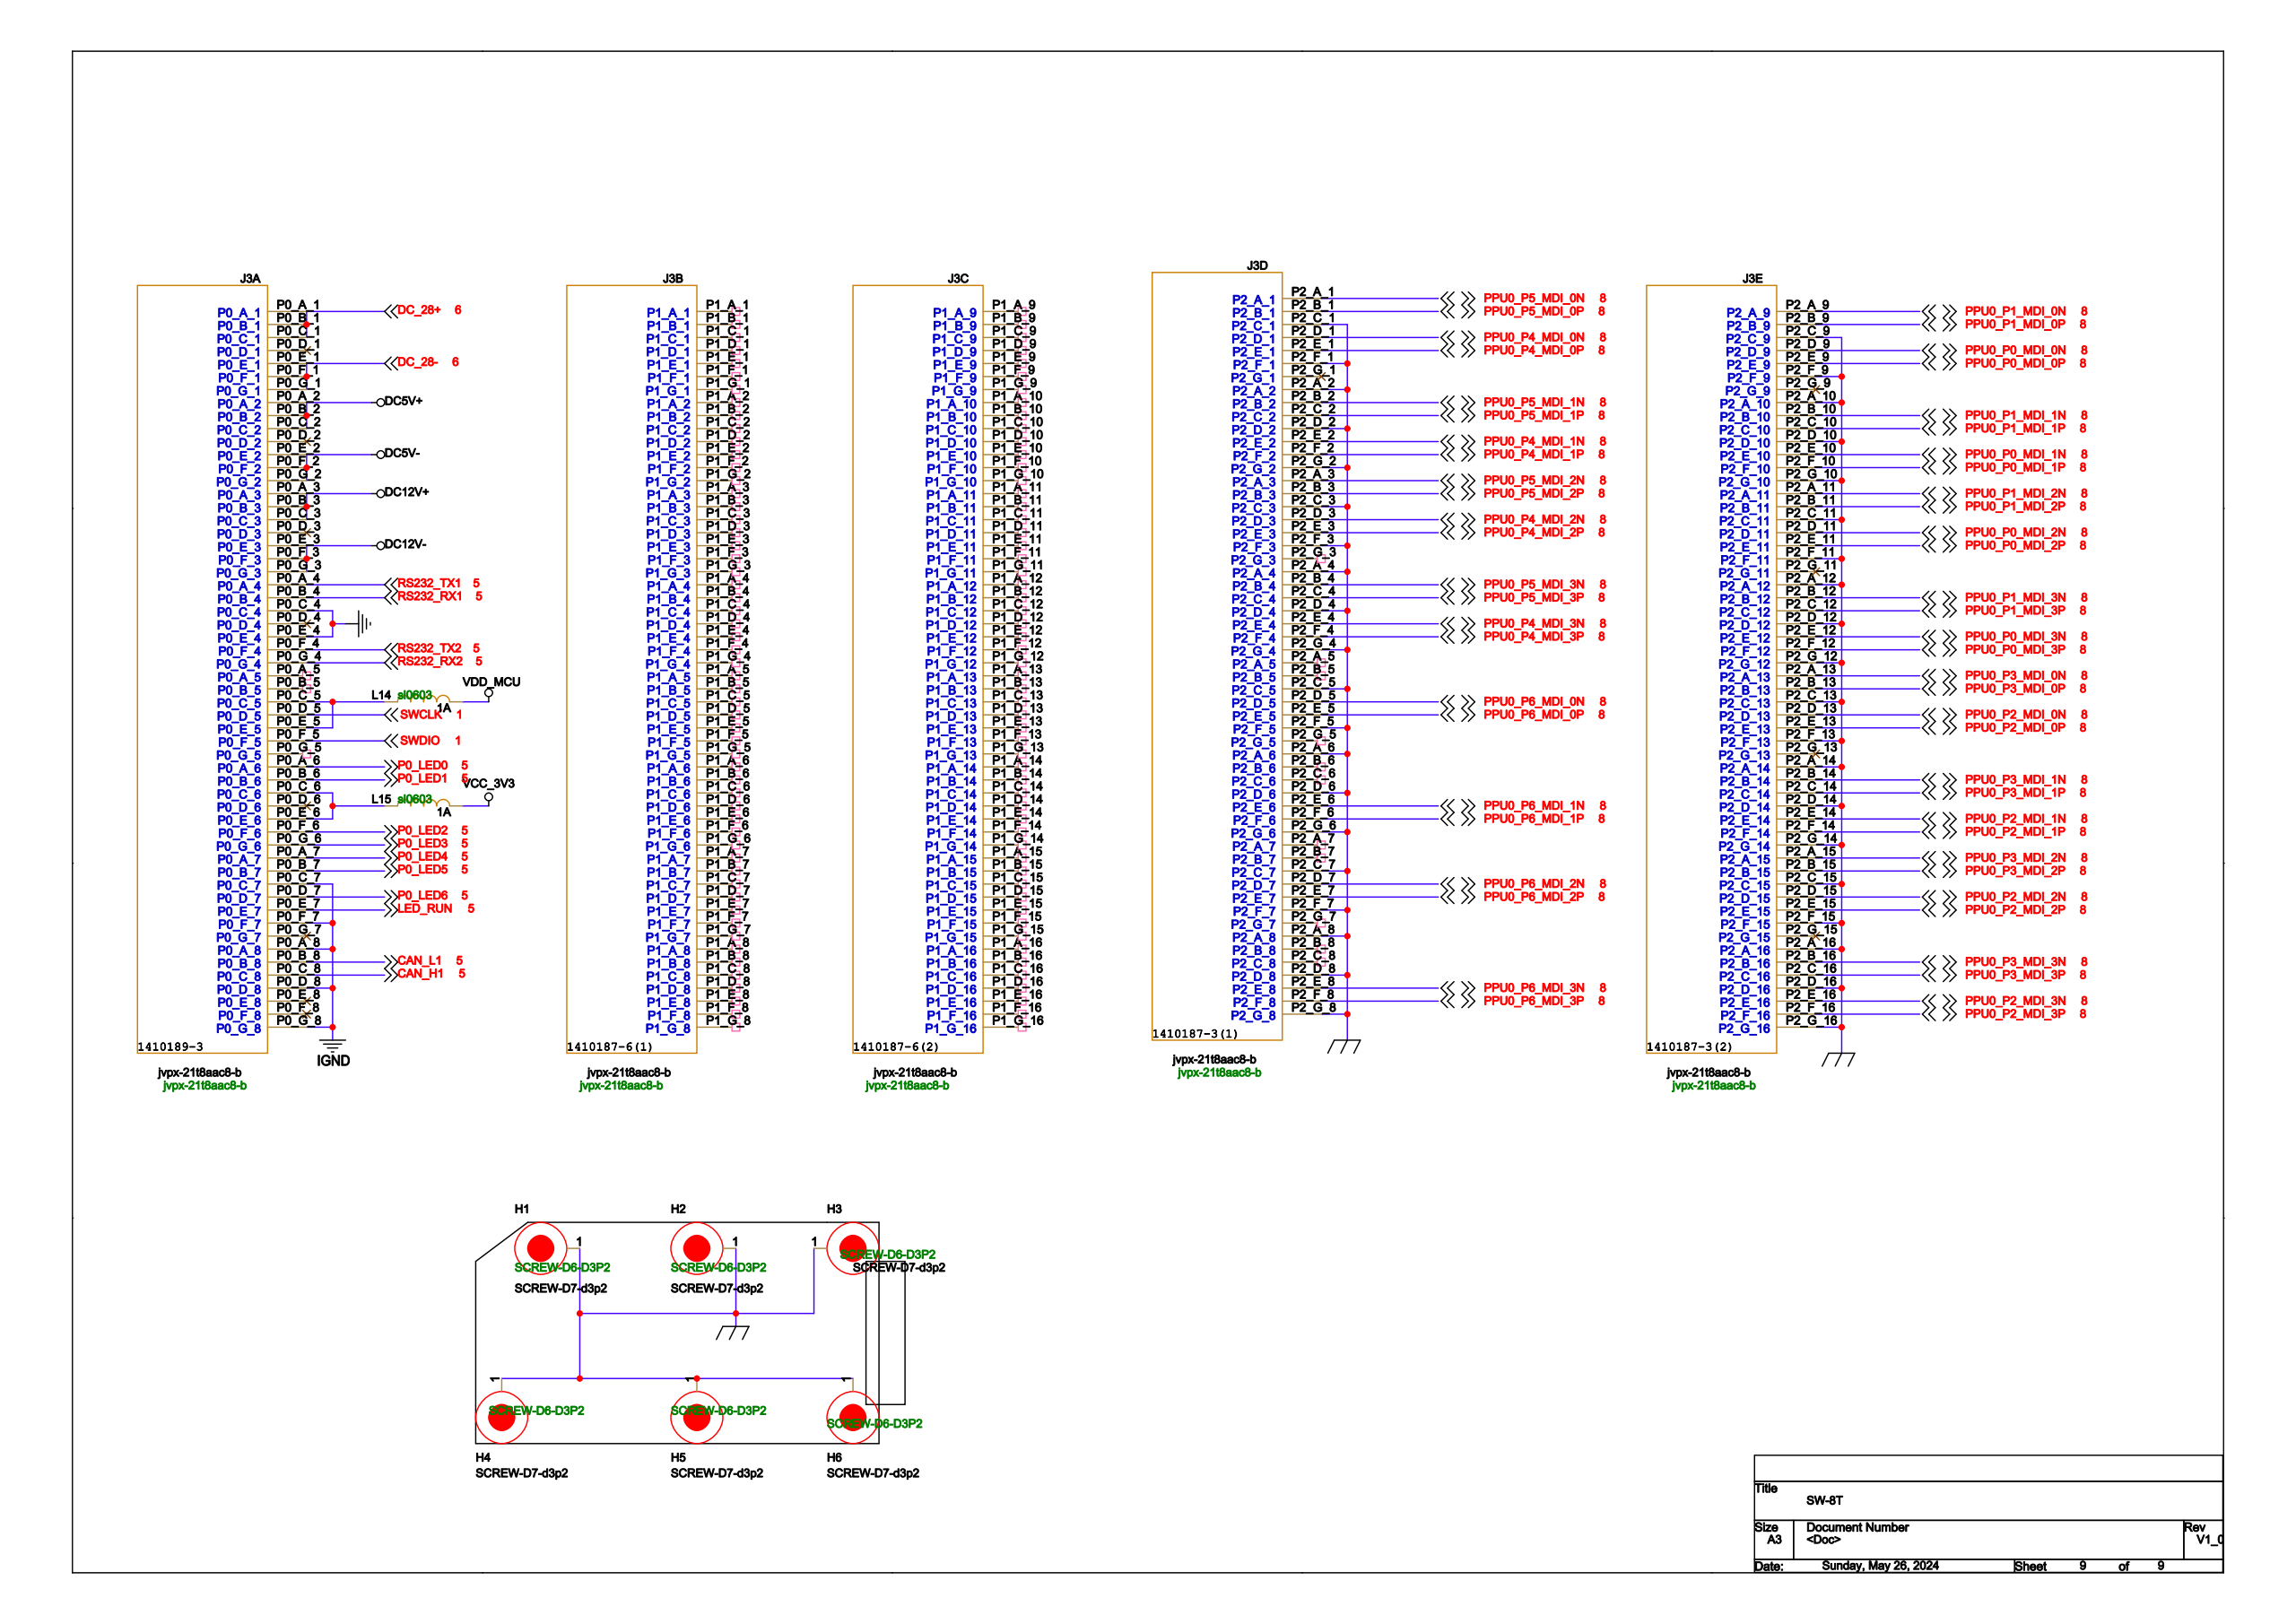Circuit board | Cadence Allegro | 399 parts | 387 nets | one sheet of the schematic
Parts on this sheet (reference | value | footprint):
H1 | SCREW-D7-d3p2 | SCREW-D6-D3P2
H2 | SCREW-D7-d3p2 | SCREW-D6-D3P2
H3 | SCREW-D7-d3p2 | SCREW-D6-D3P2
H4 | SCREW-D7-d3p2 | SCREW-D6-D3P2
H5 | SCREW-D7-d3p2 | SCREW-D6-D3P2
H6 | SCREW-D7-d3p2 | SCREW-D6-D3P2
J3 | jvpx-21t8aac8-b | JVPX-21T8AAC8-B
L14 | 1A | SL0603
L15 | 1A | SL0603
Nets of these parts (net: part-pin ...):
RS232_RX1: J3-P0_B_4
RS232_RX2: J3-P0_G_4
RS232_TX1: J3-P0_A_4
RS232_TX2: J3-P0_F_4
VDD_MCU: L14-2
VCC_3V3: L15-2
DC_28-: J3-P0_E_1 J3-P0_F_1 J3-P0_G_1
GND_EARTH: H1-1 H2-1 H3-1 H4-1 H5-1 H6-1 J3-P2_A_2 J3-P2_A_4 J3-P2_A_6 J3-P2_A_8 J3-P2_A_10 J3-P2_A_12 J3-P2_A_14 J3-P2_A_16 J3-P2_C_1 J3-P2_C_3 J3-P2_C_5 J3-P2_C_7 J3-P2_C_9 J3-P2_C_11 J3-P2_C_13 J3-P2_C_15 J3-P2_D_2 J3-P2_D_4 J3-P2_D_6 J3-P2_D_8 J3-P2_D_10 J3-P2_D_12 J3-P2_D_14 J3-P2_D_16 J3-P2_F_1 J3-P2_F_3 J3-P2_F_5 J3-P2_F_7 J3-P2_F_9 J3-P2_F_11 J3-P2_F_13 J3-P2_F_15 J3-P2_G_2 J3-P2_G_4 J3-P2_G_6 J3-P2_G_8 J3-P2_G_10 J3-P2_G_12 J3-P2_G_14 J3-P2_G_16
DC12V+: J3-P0_A_3 J3-P0_B_3 J3-P0_C_3
DC_28+: J3-P0_A_1 J3-P0_B_1 J3-P0_C_1
SWDIO: J3-P0_F_5
SWCLK: J3-P0_D_5
P0_LED0: J3-P0_A_6
P0_LED4: J3-P0_A_7
P0_LED1: J3-P0_B_6
P0_LED5: J3-P0_B_7
CAN_L1: J3-P0_B_8
N17807212: L14-1 J3-P0_C_5 J3-P0_E_5
N17788532: L15-1 J3-P0_C_6 J3-P0_E_6
CAN_H1: J3-P0_C_8
P0_LED6: J3-P0_D_7
LED_RUN: J3-P0_E_7
P0_LED2: J3-P0_F_6
P0_LED3: J3-P0_G_6
PPU0_P5_MDI_0N: J3-P2_A_1
PPU0_P5_MDI_2N: J3-P2_A_3
PPU0_P5_MDI_0P: J3-P2_B_1
PPU0_P5_MDI_1N: J3-P2_B_2
PPU0_P5_MDI_2P: J3-P2_B_3
PPU0_P5_MDI_3N: J3-P2_B_4
PPU0_P5_MDI_1P: J3-P2_C_2
PPU0_P5_MDI_3P: J3-P2_C_4
PPU0_P4_MDI_0N: J3-P2_D_1
PPU0_P4_MDI_2N: J3-P2_D_3
PPU0_P6_MDI_0N: J3-P2_D_5
PPU0_P6_MDI_2N: J3-P2_D_7
PPU0_P4_MDI_0P: J3-P2_E_1
PPU0_P4_MDI_1N: J3-P2_E_2
PPU0_P4_MDI_2P: J3-P2_E_3
PPU0_P4_MDI_3N: J3-P2_E_4
PPU0_P6_MDI_0P: J3-P2_E_5
PPU0_P6_MDI_1N: J3-P2_E_6
PPU0_P6_MDI_2P: J3-P2_E_7
PPU0_P6_MDI_3N: J3-P2_E_8
PPU0_P4_MDI_1P: J3-P2_F_2
PPU0_P4_MDI_3P: J3-P2_F_4
PPU0_P6_MDI_1P: J3-P2_F_6
PPU0_P6_MDI_3P: J3-P2_F_8
PPU0_P1_MDI_2N: J3-P2_A_11
PPU0_P3_MDI_0N: J3-P2_A_13
PPU0_P3_MDI_2N: J3-P2_A_15
PPU0_P1_MDI_0N: J3-P2_A_9
PPU0_P1_MDI_1N: J3-P2_B_10
PPU0_P1_MDI_2P: J3-P2_B_11
PPU0_P1_MDI_3N: J3-P2_B_12
PPU0_P3_MDI_0P: J3-P2_B_13
PPU0_P3_MDI_1N: J3-P2_B_14
PPU0_P3_MDI_2P: J3-P2_B_15
PPU0_P3_MDI_3N: J3-P2_B_16
PPU0_P1_MDI_0P: J3-P2_B_9
PPU0_P1_MDI_1P: J3-P2_C_10
PPU0_P1_MDI_3P: J3-P2_C_12
PPU0_P3_MDI_1P: J3-P2_C_14
PPU0_P3_MDI_3P: J3-P2_C_16
PPU0_P0_MDI_2N: J3-P2_D_11
PPU0_P2_MDI_0N: J3-P2_D_13
PPU0_P2_MDI_2N: J3-P2_D_15
PPU0_P0_MDI_0N: J3-P2_D_9
PPU0_P0_MDI_1N: J3-P2_E_10
PPU0_P0_MDI_2P: J3-P2_E_11
PPU0_P0_MDI_3N: J3-P2_E_12
PPU0_P2_MDI_0P: J3-P2_E_13
PPU0_P2_MDI_1N: J3-P2_E_14
PPU0_P2_MDI_2P: J3-P2_E_15
PPU0_P2_MDI_3N: J3-P2_E_16
PPU0_P0_MDI_0P: J3-P2_E_9
PPU0_P0_MDI_1P: J3-P2_F_10
PPU0_P0_MDI_3P: J3-P2_F_12
PPU0_P2_MDI_1P: J3-P2_F_14
PPU0_P2_MDI_3P: J3-P2_F_16